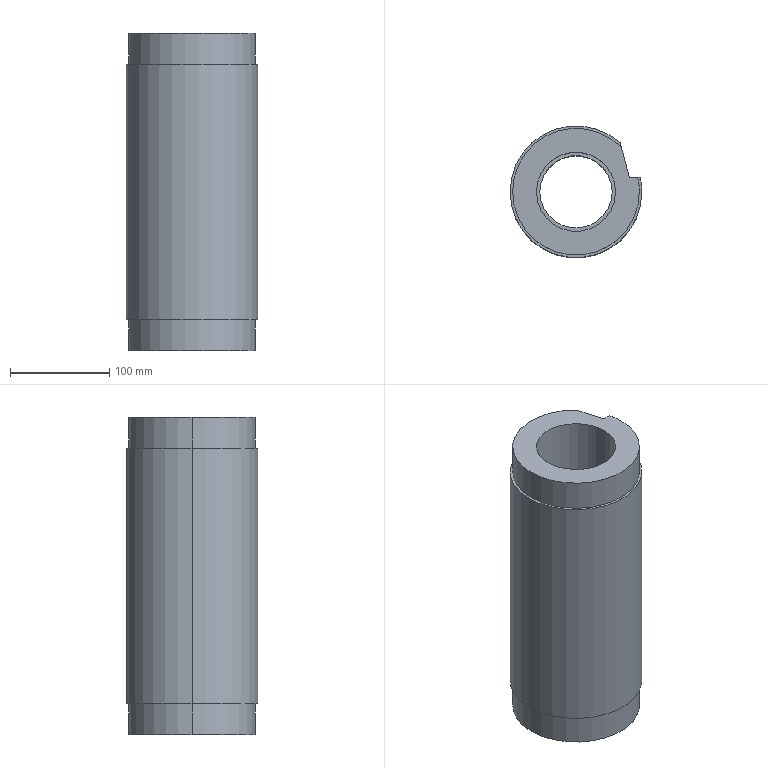Part | SolidWorks | features ICE 3, Extrusion 1, MirrorPattern 1 | 1 solid | 23 faces | box 133 x 133 x 320 mm | volume 2826163 mm3 | cylinder 15 | plane 8 | commonest cylinder face diameters 128 x6 80 x4 133 x3 73 x2
STEP:
#1=CARTESIAN_POINT('',(64.,0.,31.));
#2=VERTEX_POINT('',#1);
#3=CARTESIAN_POINT('',(62.336,14.5,31.));
#4=VERTEX_POINT('',#3);
#5=CARTESIAN_POINT('',(0.,0.,31.));
#6=DIRECTION('',(0.,0.,1.));
#7=DIRECTION('',(1.,0.,0.));
#8=AXIS2_PLACEMENT_3D('',#5,#6,#7);
#9=CIRCLE('',#8,64.);
#10=EDGE_CURVE('',#2,#4,#9,.T.);
#11=ORIENTED_EDGE('',*,*,#10,.F.);
#12=CARTESIAN_POINT('',(64.,0.,0.));
#13=VERTEX_POINT('',#12);
#14=CARTESIAN_POINT('',(64.,0.,31.));
#15=DIRECTION('',(0.,0.,-1.));
#16=VECTOR('',#15,1000.);
#17=LINE('',#14,#16);
#18=EDGE_CURVE('',#2,#13,#17,.T.);
#19=ORIENTED_EDGE('',*,*,#18,.T.);
#20=CARTESIAN_POINT('',(62.336,14.5,0.));
#21=VERTEX_POINT('',#20);
#22=CARTESIAN_POINT('',(0.,0.,0.));
#23=DIRECTION('',(0.,0.,1.));
#24=DIRECTION('',(1.,0.,0.));
#25=AXIS2_PLACEMENT_3D('',#22,#23,#24);
#26=CIRCLE('',#25,64.);
#27=EDGE_CURVE('',#13,#21,#26,.T.);
#28=ORIENTED_EDGE('',*,*,#27,.T.);
#29=CARTESIAN_POINT('',(62.336,14.5,31.));
#30=DIRECTION('',(0.,0.,1.));
#31=VECTOR('',#30,1000.);
#32=LINE('',#29,#31);
#33=EDGE_CURVE('',#21,#4,#32,.T.);
#34=ORIENTED_EDGE('',*,*,#33,.T.);
#35=EDGE_LOOP('',(#11,#19,#28,#34));
#36=FACE_OUTER_BOUND('',#35,.T.);
#37=CARTESIAN_POINT('',(0.,0.,31.));
#38=DIRECTION('',(0.,0.,-1.));
#39=DIRECTION('',(-1.,0.,0.));
#40=AXIS2_PLACEMENT_3D('',#37,#38,#39);
#41=CYLINDRICAL_SURFACE('',#40,64.);
#42=ADVANCED_FACE('',(#36),#41,.T.);
#43=ORIENTED_EDGE('',*,*,#18,.F.);
#44=CARTESIAN_POINT('',(-64.,0.,31.));
#45=VERTEX_POINT('',#44);
#46=CARTESIAN_POINT('',(0.,0.,31.));
#47=DIRECTION('',(0.,0.,1.));
#48=DIRECTION('',(1.,0.,0.));
#49=AXIS2_PLACEMENT_3D('',#46,#47,#48);
#50=CIRCLE('',#49,64.);
#51=EDGE_CURVE('',#45,#2,#50,.T.);
#52=ORIENTED_EDGE('',*,*,#51,.F.);
#53=CARTESIAN_POINT('',(-64.,0.,0.));
#54=VERTEX_POINT('',#53);
#55=CARTESIAN_POINT('',(-64.,0.,31.));
#56=DIRECTION('',(0.,0.,-1.));
#57=VECTOR('',#56,1000.);
#58=LINE('',#55,#57);
#59=EDGE_CURVE('',#45,#54,#58,.T.);
#60=ORIENTED_EDGE('',*,*,#59,.T.);
#61=CARTESIAN_POINT('',(0.,0.,0.));
#62=DIRECTION('',(0.,0.,1.));
#63=DIRECTION('',(1.,0.,0.));
#64=AXIS2_PLACEMENT_3D('',#61,#62,#63);
#65=CIRCLE('',#64,64.);
#66=EDGE_CURVE('',#54,#13,#65,.T.);
#67=ORIENTED_EDGE('',*,*,#66,.T.);
#68=EDGE_LOOP('',(#43,#52,#60,#67));
#69=FACE_OUTER_BOUND('',#68,.T.);
#70=CARTESIAN_POINT('',(0.,0.,31.));
#71=DIRECTION('',(0.,0.,-1.));
#72=DIRECTION('',(-1.,0.,0.));
#73=AXIS2_PLACEMENT_3D('',#70,#71,#72);
#74=CYLINDRICAL_SURFACE('',#73,64.);
#75=ADVANCED_FACE('',(#69),#74,.T.);
#76=CARTESIAN_POINT('',(-40.,0.,79.7));
#77=VERTEX_POINT('',#76);
#78=CARTESIAN_POINT('',(40.,0.,79.7));
#79=VERTEX_POINT('',#78);
#80=CARTESIAN_POINT('',(0.,0.,79.7));
#81=DIRECTION('',(0.,0.,1.));
#82=DIRECTION('',(1.,0.,0.));
#83=AXIS2_PLACEMENT_3D('',#80,#81,#82);
#84=CIRCLE('',#83,40.);
#85=EDGE_CURVE('',#77,#79,#84,.T.);
#86=ORIENTED_EDGE('',*,*,#85,.T.);
#87=CARTESIAN_POINT('',(40.,0.,0.));
#88=VERTEX_POINT('',#87);
#89=CARTESIAN_POINT('',(40.,0.,79.7));
#90=DIRECTION('',(0.,0.,-1.));
#91=VECTOR('',#90,1000.);
#92=LINE('',#89,#91);
#93=EDGE_CURVE('',#79,#88,#92,.T.);
#94=ORIENTED_EDGE('',*,*,#93,.T.);
#95=CARTESIAN_POINT('',(-40.,0.,0.));
#96=VERTEX_POINT('',#95);
#97=CARTESIAN_POINT('',(0.,0.,0.));
#98=DIRECTION('',(0.,0.,1.));
#99=DIRECTION('',(1.,0.,0.));
#100=AXIS2_PLACEMENT_3D('',#97,#98,#99);
#101=CIRCLE('',#100,40.);
#102=EDGE_CURVE('',#96,#88,#101,.T.);
#103=ORIENTED_EDGE('',*,*,#102,.F.);
#104=CARTESIAN_POINT('',(-40.,0.,79.7));
#105=DIRECTION('',(0.,0.,-1.));
#106=VECTOR('',#105,1000.);
#107=LINE('',#104,#106);
#108=EDGE_CURVE('',#77,#96,#107,.T.);
#109=ORIENTED_EDGE('',*,*,#108,.F.);
#110=EDGE_LOOP('',(#86,#94,#103,#109));
#111=FACE_OUTER_BOUND('',#110,.T.);
#112=CARTESIAN_POINT('',(0.,0.,79.7));
#113=DIRECTION('',(0.,0.,-1.));
#114=DIRECTION('',(-1.,0.,0.));
#115=AXIS2_PLACEMENT_3D('',#112,#113,#114);
#116=CYLINDRICAL_SURFACE('',#115,40.);
#117=ADVANCED_FACE('',(#111),#116,.F.);
#118=CARTESIAN_POINT('',(45.81,44.693,289.));
#119=VERTEX_POINT('',#118);
#120=CARTESIAN_POINT('',(-64.,0.,289.));
#121=VERTEX_POINT('',#120);
#122=CARTESIAN_POINT('',(0.,0.,289.));
#123=DIRECTION('',(0.,0.,1.));
#124=DIRECTION('',(1.,0.,0.));
#125=AXIS2_PLACEMENT_3D('',#122,#123,#124);
#126=CIRCLE('',#125,64.);
#127=EDGE_CURVE('',#119,#121,#126,.T.);
#128=ORIENTED_EDGE('',*,*,#127,.T.);
#129=CARTESIAN_POINT('',(-64.,0.,320.));
#130=VERTEX_POINT('',#129);
#131=CARTESIAN_POINT('',(-64.,0.,289.));
#132=DIRECTION('',(0.,0.,1.));
#133=VECTOR('',#132,1000.);
#134=LINE('',#131,#133);
#135=EDGE_CURVE('',#121,#130,#134,.T.);
#136=ORIENTED_EDGE('',*,*,#135,.T.);
#137=CARTESIAN_POINT('',(45.81,44.693,320.));
#138=VERTEX_POINT('',#137);
#139=CARTESIAN_POINT('',(0.,0.,320.));
#140=DIRECTION('',(0.,0.,1.));
#141=DIRECTION('',(1.,0.,0.));
#142=AXIS2_PLACEMENT_3D('',#139,#140,#141);
#143=CIRCLE('',#142,64.);
#144=EDGE_CURVE('',#138,#130,#143,.T.);
#145=ORIENTED_EDGE('',*,*,#144,.F.);
#146=CARTESIAN_POINT('',(45.81,44.693,289.));
#147=DIRECTION('',(0.,0.,1.));
#148=VECTOR('',#147,1000.);
#149=LINE('',#146,#148);
#150=EDGE_CURVE('',#119,#138,#149,.T.);
#151=ORIENTED_EDGE('',*,*,#150,.F.);
#152=EDGE_LOOP('',(#128,#136,#145,#151));
#153=FACE_OUTER_BOUND('',#152,.T.);
#154=CARTESIAN_POINT('',(0.,0.,289.));
#155=DIRECTION('',(0.,0.,1.));
#156=DIRECTION('',(1.,0.,0.));
#157=AXIS2_PLACEMENT_3D('',#154,#155,#156);
#158=CYLINDRICAL_SURFACE('',#157,64.);
#159=ADVANCED_FACE('',(#153),#158,.T.);
#160=ORIENTED_EDGE('',*,*,#135,.F.);
#161=CARTESIAN_POINT('',(64.,0.,289.));
#162=VERTEX_POINT('',#161);
#163=CARTESIAN_POINT('',(0.,0.,289.));
#164=DIRECTION('',(0.,0.,1.));
#165=DIRECTION('',(1.,0.,0.));
#166=AXIS2_PLACEMENT_3D('',#163,#164,#165);
#167=CIRCLE('',#166,64.);
#168=EDGE_CURVE('',#121,#162,#167,.T.);
#169=ORIENTED_EDGE('',*,*,#168,.T.);
#170=CARTESIAN_POINT('',(64.,0.,320.));
#171=VERTEX_POINT('',#170);
#172=CARTESIAN_POINT('',(64.,0.,289.));
#173=DIRECTION('',(0.,0.,1.));
#174=VECTOR('',#173,1000.);
#175=LINE('',#172,#174);
#176=EDGE_CURVE('',#162,#171,#175,.T.);
#177=ORIENTED_EDGE('',*,*,#176,.T.);
#178=CARTESIAN_POINT('',(0.,0.,320.));
#179=DIRECTION('',(0.,0.,1.));
#180=DIRECTION('',(1.,0.,0.));
#181=AXIS2_PLACEMENT_3D('',#178,#179,#180);
#182=CIRCLE('',#181,64.);
#183=EDGE_CURVE('',#130,#171,#182,.T.);
#184=ORIENTED_EDGE('',*,*,#183,.F.);
#185=EDGE_LOOP('',(#160,#169,#177,#184));
#186=FACE_OUTER_BOUND('',#185,.T.);
#187=CARTESIAN_POINT('',(0.,0.,289.));
#188=DIRECTION('',(0.,0.,1.));
#189=DIRECTION('',(1.,0.,0.));
#190=AXIS2_PLACEMENT_3D('',#187,#188,#189);
#191=CYLINDRICAL_SURFACE('',#190,64.);
#192=ADVANCED_FACE('',(#186),#191,.T.);
#193=CARTESIAN_POINT('',(-40.,0.,240.3));
#194=VERTEX_POINT('',#193);
#195=CARTESIAN_POINT('',(40.,0.,240.3));
#196=VERTEX_POINT('',#195);
#197=CARTESIAN_POINT('',(0.,0.,240.3));
#198=DIRECTION('',(0.,0.,1.));
#199=DIRECTION('',(1.,0.,0.));
#200=AXIS2_PLACEMENT_3D('',#197,#198,#199);
#201=CIRCLE('',#200,40.);
#202=EDGE_CURVE('',#194,#196,#201,.T.);
#203=ORIENTED_EDGE('',*,*,#202,.F.);
#204=CARTESIAN_POINT('',(-40.,0.,320.));
#205=VERTEX_POINT('',#204);
#206=CARTESIAN_POINT('',(-40.,0.,240.3));
#207=DIRECTION('',(0.,0.,1.));
#208=VECTOR('',#207,1000.);
#209=LINE('',#206,#208);
#210=EDGE_CURVE('',#194,#205,#209,.T.);
#211=ORIENTED_EDGE('',*,*,#210,.T.);
#212=CARTESIAN_POINT('',(40.,0.,320.));
#213=VERTEX_POINT('',#212);
#214=CARTESIAN_POINT('',(0.,0.,320.));
#215=DIRECTION('',(0.,0.,1.));
#216=DIRECTION('',(1.,0.,0.));
#217=AXIS2_PLACEMENT_3D('',#214,#215,#216);
#218=CIRCLE('',#217,40.);
#219=EDGE_CURVE('',#205,#213,#218,.T.);
#220=ORIENTED_EDGE('',*,*,#219,.T.);
#221=CARTESIAN_POINT('',(40.,0.,240.3));
#222=DIRECTION('',(0.,0.,1.));
#223=VECTOR('',#222,1000.);
#224=LINE('',#221,#223);
#225=EDGE_CURVE('',#196,#213,#224,.T.);
#226=ORIENTED_EDGE('',*,*,#225,.F.);
#227=EDGE_LOOP('',(#203,#211,#220,#226));
#228=FACE_OUTER_BOUND('',#227,.T.);
#229=CARTESIAN_POINT('',(0.,0.,240.3));
#230=DIRECTION('',(0.,0.,1.));
#231=DIRECTION('',(1.,0.,0.));
#232=AXIS2_PLACEMENT_3D('',#229,#230,#231);
#233=CYLINDRICAL_SURFACE('',#232,40.);
#234=ADVANCED_FACE('',(#228),#233,.F.);
#235=CARTESIAN_POINT('',(-36.5,0.,240.3));
#236=VERTEX_POINT('',#235);
#237=CARTESIAN_POINT('',(36.5,0.,240.3));
#238=VERTEX_POINT('',#237);
#239=CARTESIAN_POINT('',(0.,0.,240.3));
#240=DIRECTION('',(0.,0.,1.));
#241=DIRECTION('',(1.,0.,0.));
#242=AXIS2_PLACEMENT_3D('',#239,#240,#241);
#243=CIRCLE('',#242,36.5);
#244=EDGE_CURVE('',#236,#238,#243,.T.);
#245=ORIENTED_EDGE('',*,*,#244,.T.);
#246=CARTESIAN_POINT('',(36.5,0.,79.7));
#247=VERTEX_POINT('',#246);
#248=CARTESIAN_POINT('',(36.5,0.,320.));
#249=DIRECTION('',(0.,0.,-1.));
#250=VECTOR('',#249,1000.);
#251=LINE('',#248,#250);
#252=EDGE_CURVE('',#238,#247,#251,.T.);
#253=ORIENTED_EDGE('',*,*,#252,.T.);
#254=CARTESIAN_POINT('',(-36.5,0.,79.7));
#255=VERTEX_POINT('',#254);
#256=CARTESIAN_POINT('',(0.,0.,79.7));
#257=DIRECTION('',(0.,0.,-1.));
#258=DIRECTION('',(-1.,0.,0.));
#259=AXIS2_PLACEMENT_3D('',#256,#257,#258);
#260=CIRCLE('',#259,36.5);
#261=EDGE_CURVE('',#247,#255,#260,.T.);
#262=ORIENTED_EDGE('',*,*,#261,.T.);
#263=CARTESIAN_POINT('',(-36.5,0.,320.));
#264=DIRECTION('',(0.,0.,-1.));
#265=VECTOR('',#264,1000.);
#266=LINE('',#263,#265);
#267=EDGE_CURVE('',#236,#255,#266,.T.);
#268=ORIENTED_EDGE('',*,*,#267,.F.);
#269=EDGE_LOOP('',(#245,#253,#262,#268));
#270=FACE_OUTER_BOUND('',#269,.T.);
#271=CARTESIAN_POINT('',(0.,0.,320.));
#272=DIRECTION('',(0.,0.,-1.));
#273=DIRECTION('',(-1.,0.,0.));
#274=AXIS2_PLACEMENT_3D('',#271,#272,#273);
#275=CYLINDRICAL_SURFACE('',#274,36.5);
#276=ADVANCED_FACE('',(#270),#275,.F.);
#277=CARTESIAN_POINT('',(66.5,0.,289.));
#278=VERTEX_POINT('',#277);
#279=CARTESIAN_POINT('',(64.9,14.5,289.));
#280=VERTEX_POINT('',#279);
#281=CARTESIAN_POINT('',(0.,0.,289.));
#282=DIRECTION('',(0.,0.,1.));
#283=DIRECTION('',(1.,0.,0.));
#284=AXIS2_PLACEMENT_3D('',#281,#282,#283);
#285=CIRCLE('',#284,66.5);
#286=EDGE_CURVE('',#278,#280,#285,.T.);
#287=ORIENTED_EDGE('',*,*,#286,.F.);
#288=CARTESIAN_POINT('',(66.5,0.,31.));
#289=VERTEX_POINT('',#288);
#290=CARTESIAN_POINT('',(66.5,0.,320.));
#291=DIRECTION('',(0.,0.,-1.));
#292=VECTOR('',#291,1000.);
#293=LINE('',#290,#292);
#294=EDGE_CURVE('',#278,#289,#293,.T.);
#295=ORIENTED_EDGE('',*,*,#294,.T.);
#296=CARTESIAN_POINT('',(64.9,14.5,31.));
#297=VERTEX_POINT('',#296);
#298=CARTESIAN_POINT('',(0.,0.,31.));
#299=DIRECTION('',(0.,0.,1.));
#300=DIRECTION('',(1.,0.,0.));
#301=AXIS2_PLACEMENT_3D('',#298,#299,#300);
#302=CIRCLE('',#301,66.5);
#303=EDGE_CURVE('',#289,#297,#302,.T.);
#304=ORIENTED_EDGE('',*,*,#303,.T.);
#305=CARTESIAN_POINT('',(64.9,14.5,0.));
#306=DIRECTION('',(0.,0.,1.));
#307=VECTOR('',#306,1000.);
#308=LINE('',#305,#307);
#309=EDGE_CURVE('',#297,#280,#308,.T.);
#310=ORIENTED_EDGE('',*,*,#309,.T.);
#311=EDGE_LOOP('',(#287,#295,#304,#310));
#312=FACE_OUTER_BOUND('',#311,.T.);
#313=CARTESIAN_POINT('',(0.,0.,320.));
#314=DIRECTION('',(0.,0.,-1.));
#315=DIRECTION('',(-1.,0.,0.));
#316=AXIS2_PLACEMENT_3D('',#313,#314,#315);
#317=CYLINDRICAL_SURFACE('',#316,66.5);
#318=ADVANCED_FACE('',(#312),#317,.T.);
#319=ORIENTED_EDGE('',*,*,#294,.F.);
#320=CARTESIAN_POINT('',(-66.5,0.,289.));
#321=VERTEX_POINT('',#320);
#322=CARTESIAN_POINT('',(0.,0.,289.));
#323=DIRECTION('',(0.,0.,1.));
#324=DIRECTION('',(1.,0.,0.));
#325=AXIS2_PLACEMENT_3D('',#322,#323,#324);
#326=CIRCLE('',#325,66.5);
#327=EDGE_CURVE('',#321,#278,#326,.T.);
#328=ORIENTED_EDGE('',*,*,#327,.F.);
#329=CARTESIAN_POINT('',(-66.5,0.,31.));
#330=VERTEX_POINT('',#329);
#331=CARTESIAN_POINT('',(-66.5,0.,320.));
#332=DIRECTION('',(0.,0.,-1.));
#333=VECTOR('',#332,1000.);
#334=LINE('',#331,#333);
#335=EDGE_CURVE('',#321,#330,#334,.T.);
#336=ORIENTED_EDGE('',*,*,#335,.T.);
#337=CARTESIAN_POINT('',(0.,0.,31.));
#338=DIRECTION('',(0.,0.,1.));
#339=DIRECTION('',(1.,0.,0.));
#340=AXIS2_PLACEMENT_3D('',#337,#338,#339);
#341=CIRCLE('',#340,66.5);
#342=EDGE_CURVE('',#330,#289,#341,.T.);
#343=ORIENTED_EDGE('',*,*,#342,.T.);
#344=EDGE_LOOP('',(#319,#328,#336,#343));
#345=FACE_OUTER_BOUND('',#344,.T.);
#346=CARTESIAN_POINT('',(0.,0.,320.));
#347=DIRECTION('',(0.,0.,-1.));
#348=DIRECTION('',(-1.,0.,0.));
#349=AXIS2_PLACEMENT_3D('',#346,#347,#348);
#350=CYLINDRICAL_SURFACE('',#349,66.5);
#351=ADVANCED_FACE('',(#345),#350,.T.);
#352=ORIENTED_EDGE('',*,*,#335,.F.);
#353=CARTESIAN_POINT('',(44.558,49.364,289.));
#354=VERTEX_POINT('',#353);
#355=CARTESIAN_POINT('',(0.,0.,289.));
#356=DIRECTION('',(0.,0.,1.));
#357=DIRECTION('',(1.,0.,0.));
#358=AXIS2_PLACEMENT_3D('',#355,#356,#357);
#359=CIRCLE('',#358,66.5);
#360=EDGE_CURVE('',#354,#321,#359,.T.);
#361=ORIENTED_EDGE('',*,*,#360,.F.);
#362=CARTESIAN_POINT('',(44.558,49.364,31.));
#363=VERTEX_POINT('',#362);
#364=CARTESIAN_POINT('',(44.558,49.364,0.));
#365=DIRECTION('',(0.,0.,1.));
#366=VECTOR('',#365,1000.);
#367=LINE('',#364,#366);
#368=EDGE_CURVE('',#363,#354,#367,.T.);
#369=ORIENTED_EDGE('',*,*,#368,.F.);
#370=CARTESIAN_POINT('',(0.,0.,31.));
#371=DIRECTION('',(0.,0.,1.));
#372=DIRECTION('',(1.,0.,0.));
#373=AXIS2_PLACEMENT_3D('',#370,#371,#372);
#374=CIRCLE('',#373,66.5);
#375=EDGE_CURVE('',#363,#330,#374,.T.);
#376=ORIENTED_EDGE('',*,*,#375,.T.);
#377=EDGE_LOOP('',(#352,#361,#369,#376));
#378=FACE_OUTER_BOUND('',#377,.T.);
#379=CARTESIAN_POINT('',(0.,0.,320.));
#380=DIRECTION('',(0.,0.,-1.));
#381=DIRECTION('',(-1.,0.,0.));
#382=AXIS2_PLACEMENT_3D('',#379,#380,#381);
#383=CYLINDRICAL_SURFACE('',#382,66.5);
#384=ADVANCED_FACE('',(#378),#383,.T.);
#385=ORIENTED_EDGE('',*,*,#252,.F.);
#386=CARTESIAN_POINT('',(0.,0.,240.3));
#387=DIRECTION('',(0.,0.,1.));
#388=DIRECTION('',(1.,0.,0.));
#389=AXIS2_PLACEMENT_3D('',#386,#387,#388);
#390=CIRCLE('',#389,36.5);
#391=EDGE_CURVE('',#238,#236,#390,.T.);
#392=ORIENTED_EDGE('',*,*,#391,.T.);
#393=ORIENTED_EDGE('',*,*,#267,.T.);
#394=CARTESIAN_POINT('',(0.,0.,79.7));
#395=DIRECTION('',(0.,0.,-1.));
#396=DIRECTION('',(-1.,0.,0.));
#397=AXIS2_PLACEMENT_3D('',#394,#395,#396);
#398=CIRCLE('',#397,36.5);
#399=EDGE_CURVE('',#255,#247,#398,.T.);
#400=ORIENTED_EDGE('',*,*,#399,.T.);
#401=EDGE_LOOP('',(#385,#392,#393,#400));
#402=FACE_OUTER_BOUND('',#401,.T.);
#403=CARTESIAN_POINT('',(0.,0.,320.));
#404=DIRECTION('',(0.,0.,-1.));
#405=DIRECTION('',(-1.,0.,0.));
#406=AXIS2_PLACEMENT_3D('',#403,#404,#405);
#407=CYLINDRICAL_SURFACE('',#406,36.5);
#408=ADVANCED_FACE('',(#402),#407,.F.);
#409=CARTESIAN_POINT('',(45.81,44.693,0.));
#410=VERTEX_POINT('',#409);
#411=CARTESIAN_POINT('',(53.9,14.5,0.));
#412=VERTEX_POINT('',#411);
#413=CARTESIAN_POINT('',(53.9,14.5,0.));
#414=DIRECTION('',(0.2588,-0.9659,0.));
#415=VECTOR('',#414,1000.);
#416=LINE('',#413,#415);
#417=EDGE_CURVE('',#410,#412,#416,.T.);
#418=ORIENTED_EDGE('',*,*,#417,.T.);
#419=CARTESIAN_POINT('',(64.9,14.5,0.));
#420=DIRECTION('',(1.,0.,0.));
#421=VECTOR('',#420,1000.);
#422=LINE('',#419,#421);
#423=EDGE_CURVE('',#412,#21,#422,.T.);
#424=ORIENTED_EDGE('',*,*,#423,.T.);
#425=ORIENTED_EDGE('',*,*,#27,.F.);
#426=ORIENTED_EDGE('',*,*,#66,.F.);
#427=CARTESIAN_POINT('',(0.,0.,0.));
#428=DIRECTION('',(0.,0.,1.));
#429=DIRECTION('',(1.,0.,0.));
#430=AXIS2_PLACEMENT_3D('',#427,#428,#429);
#431=CIRCLE('',#430,64.);
#432=EDGE_CURVE('',#410,#54,#431,.T.);
#433=ORIENTED_EDGE('',*,*,#432,.F.);
#434=EDGE_LOOP('',(#418,#424,#425,#426,#433));
#435=FACE_OUTER_BOUND('',#434,.T.);
#436=ORIENTED_EDGE('',*,*,#102,.T.);
#437=CARTESIAN_POINT('',(0.,0.,0.));
#438=DIRECTION('',(0.,0.,1.));
#439=DIRECTION('',(1.,0.,0.));
#440=AXIS2_PLACEMENT_3D('',#437,#438,#439);
#441=CIRCLE('',#440,40.);
#442=EDGE_CURVE('',#88,#96,#441,.T.);
#443=ORIENTED_EDGE('',*,*,#442,.T.);
#444=EDGE_LOOP('',(#436,#443));
#445=FACE_BOUND('',#444,.T.);
#446=CARTESIAN_POINT('',(0.,0.,0.));
#447=DIRECTION('',(0.,0.,1.));
#448=DIRECTION('',(1.,0.,0.));
#449=AXIS2_PLACEMENT_3D('',#446,#447,#448);
#450=PLANE('',#449);
#451=ADVANCED_FACE('',(#435,#445),#450,.F.);
#452=CARTESIAN_POINT('',(53.9,14.5,320.));
#453=VERTEX_POINT('',#452);
#454=CARTESIAN_POINT('',(62.336,14.5,320.));
#455=VERTEX_POINT('',#454);
#456=CARTESIAN_POINT('',(64.9,14.5,320.));
#457=DIRECTION('',(1.,0.,0.));
#458=VECTOR('',#457,1000.);
#459=LINE('',#456,#458);
#460=EDGE_CURVE('',#453,#455,#459,.T.);
#461=ORIENTED_EDGE('',*,*,#460,.F.);
#462=CARTESIAN_POINT('',(53.9,14.5,320.));
#463=DIRECTION('',(0.2588,-0.9659,0.));
#464=VECTOR('',#463,1000.);
#465=LINE('',#462,#464);
#466=EDGE_CURVE('',#138,#453,#465,.T.);
#467=ORIENTED_EDGE('',*,*,#466,.F.);
#468=ORIENTED_EDGE('',*,*,#144,.T.);
#469=ORIENTED_EDGE('',*,*,#183,.T.);
#470=CARTESIAN_POINT('',(0.,0.,320.));
#471=DIRECTION('',(0.,0.,1.));
#472=DIRECTION('',(1.,0.,0.));
#473=AXIS2_PLACEMENT_3D('',#470,#471,#472);
#474=CIRCLE('',#473,64.);
#475=EDGE_CURVE('',#171,#455,#474,.T.);
#476=ORIENTED_EDGE('',*,*,#475,.T.);
#477=EDGE_LOOP('',(#461,#467,#468,#469,#476));
#478=FACE_OUTER_BOUND('',#477,.T.);
#479=CARTESIAN_POINT('',(0.,0.,320.));
#480=DIRECTION('',(0.,0.,1.));
#481=DIRECTION('',(1.,0.,0.));
#482=AXIS2_PLACEMENT_3D('',#479,#480,#481);
#483=CIRCLE('',#482,40.);
#484=EDGE_CURVE('',#213,#205,#483,.T.);
#485=ORIENTED_EDGE('',*,*,#484,.F.);
#486=ORIENTED_EDGE('',*,*,#219,.F.);
#487=EDGE_LOOP('',(#485,#486));
#488=FACE_BOUND('',#487,.T.);
#489=CARTESIAN_POINT('',(0.,0.,320.));
#490=DIRECTION('',(0.,0.,1.));
#491=DIRECTION('',(1.,0.,0.));
#492=AXIS2_PLACEMENT_3D('',#489,#490,#491);
#493=PLANE('',#492);
#494=ADVANCED_FACE('',(#478,#488),#493,.T.);
#495=ORIENTED_EDGE('',*,*,#210,.F.);
#496=CARTESIAN_POINT('',(0.,0.,240.3));
#497=DIRECTION('',(0.,0.,1.));
#498=DIRECTION('',(1.,0.,0.));
#499=AXIS2_PLACEMENT_3D('',#496,#497,#498);
#500=CIRCLE('',#499,40.);
#501=EDGE_CURVE('',#196,#194,#500,.T.);
#502=ORIENTED_EDGE('',*,*,#501,.F.);
#503=ORIENTED_EDGE('',*,*,#225,.T.);
#504=ORIENTED_EDGE('',*,*,#484,.T.);
#505=EDGE_LOOP('',(#495,#502,#503,#504));
#506=FACE_OUTER_BOUND('',#505,.T.);
#507=CARTESIAN_POINT('',(0.,0.,240.3));
#508=DIRECTION('',(0.,0.,1.));
#509=DIRECTION('',(1.,0.,0.));
#510=AXIS2_PLACEMENT_3D('',#507,#508,#509);
#511=CYLINDRICAL_SURFACE('',#510,40.);
#512=ADVANCED_FACE('',(#506),#511,.F.);
#513=ORIENTED_EDGE('',*,*,#244,.F.);
#514=ORIENTED_EDGE('',*,*,#391,.F.);
#515=EDGE_LOOP('',(#513,#514));
#516=FACE_BOUND('',#515,.T.);
#517=ORIENTED_EDGE('',*,*,#501,.T.);
#518=ORIENTED_EDGE('',*,*,#202,.T.);
#519=EDGE_LOOP('',(#517,#518));
#520=FACE_OUTER_BOUND('',#519,.T.);
#521=CARTESIAN_POINT('',(0.,0.,240.3));
#522=DIRECTION('',(0.,0.,1.));
#523=DIRECTION('',(1.,0.,0.));
#524=AXIS2_PLACEMENT_3D('',#521,#522,#523);
#525=PLANE('',#524);
#526=ADVANCED_FACE('',(#516,#520),#525,.T.);
#527=CARTESIAN_POINT('',(62.336,14.5,289.));
#528=VERTEX_POINT('',#527);
#529=CARTESIAN_POINT('',(0.,14.5,289.));
#530=DIRECTION('',(1.,0.,0.));
#531=VECTOR('',#530,1000.);
#532=LINE('',#529,#531);
#533=EDGE_CURVE('',#528,#280,#532,.T.);
#534=ORIENTED_EDGE('',*,*,#533,.F.);
#535=CARTESIAN_POINT('',(0.,0.,289.));
#536=DIRECTION('',(0.,0.,1.));
#537=DIRECTION('',(1.,0.,0.));
#538=AXIS2_PLACEMENT_3D('',#535,#536,#537);
#539=CIRCLE('',#538,64.);
#540=EDGE_CURVE('',#162,#528,#539,.T.);
#541=ORIENTED_EDGE('',*,*,#540,.F.);
#542=ORIENTED_EDGE('',*,*,#168,.F.);
#543=ORIENTED_EDGE('',*,*,#127,.F.);
#544=CARTESIAN_POINT('',(53.914,14.446,289.));
#545=DIRECTION('',(0.2588,-0.9659,0.));
#546=VECTOR('',#545,1000.);
#547=LINE('',#544,#546);
#548=EDGE_CURVE('',#354,#119,#547,.T.);
#549=ORIENTED_EDGE('',*,*,#548,.F.);
#550=ORIENTED_EDGE('',*,*,#360,.T.);
#551=ORIENTED_EDGE('',*,*,#327,.T.);
#552=ORIENTED_EDGE('',*,*,#286,.T.);
#553=EDGE_LOOP('',(#534,#541,#542,#543,#549,#550,#551,#552));
#554=FACE_OUTER_BOUND('',#553,.T.);
#555=CARTESIAN_POINT('',(0.,0.,289.));
#556=DIRECTION('',(0.,0.,1.));
#557=DIRECTION('',(1.,0.,0.));
#558=AXIS2_PLACEMENT_3D('',#555,#556,#557);
#559=PLANE('',#558);
#560=ADVANCED_FACE('',(#554),#559,.T.);
#561=ORIENTED_EDGE('',*,*,#176,.F.);
#562=ORIENTED_EDGE('',*,*,#540,.T.);
#563=CARTESIAN_POINT('',(62.336,14.5,289.));
#564=DIRECTION('',(0.,0.,-1.));
#565=VECTOR('',#564,1000.);
#566=LINE('',#563,#565);
#567=EDGE_CURVE('',#455,#528,#566,.T.);
#568=ORIENTED_EDGE('',*,*,#567,.F.);
#569=ORIENTED_EDGE('',*,*,#475,.F.);
#570=EDGE_LOOP('',(#561,#562,#568,#569));
#571=FACE_OUTER_BOUND('',#570,.T.);
#572=CARTESIAN_POINT('',(0.,0.,289.));
#573=DIRECTION('',(0.,0.,1.));
#574=DIRECTION('',(1.,0.,0.));
#575=AXIS2_PLACEMENT_3D('',#572,#573,#574);
#576=CYLINDRICAL_SURFACE('',#575,64.);
#577=ADVANCED_FACE('',(#571),#576,.T.);
#578=ORIENTED_EDGE('',*,*,#93,.F.);
#579=CARTESIAN_POINT('',(0.,0.,79.7));
#580=DIRECTION('',(0.,0.,1.));
#581=DIRECTION('',(1.,0.,0.));
#582=AXIS2_PLACEMENT_3D('',#579,#580,#581);
#583=CIRCLE('',#582,40.);
#584=EDGE_CURVE('',#79,#77,#583,.T.);
#585=ORIENTED_EDGE('',*,*,#584,.T.);
#586=ORIENTED_EDGE('',*,*,#108,.T.);
#587=ORIENTED_EDGE('',*,*,#442,.F.);
#588=EDGE_LOOP('',(#578,#585,#586,#587));
#589=FACE_OUTER_BOUND('',#588,.T.);
#590=CARTESIAN_POINT('',(0.,0.,79.7));
#591=DIRECTION('',(0.,0.,-1.));
#592=DIRECTION('',(-1.,0.,0.));
#593=AXIS2_PLACEMENT_3D('',#590,#591,#592);
#594=CYLINDRICAL_SURFACE('',#593,40.);
#595=ADVANCED_FACE('',(#589),#594,.F.);
#596=ORIENTED_EDGE('',*,*,#399,.F.);
#597=ORIENTED_EDGE('',*,*,#261,.F.);
#598=EDGE_LOOP('',(#596,#597));
#599=FACE_BOUND('',#598,.T.);
#600=ORIENTED_EDGE('',*,*,#85,.F.);
#601=ORIENTED_EDGE('',*,*,#584,.F.);
#602=EDGE_LOOP('',(#600,#601));
#603=FACE_OUTER_BOUND('',#602,.T.);
#604=CARTESIAN_POINT('',(0.,0.,79.7));
#605=DIRECTION('',(0.,0.,-1.));
#606=DIRECTION('',(1.,0.,0.));
#607=AXIS2_PLACEMENT_3D('',#604,#605,#606);
#608=PLANE('',#607);
#609=ADVANCED_FACE('',(#599,#603),#608,.T.);
#610=CARTESIAN_POINT('',(0.,14.5,31.));
#611=DIRECTION('',(-1.,0.,0.));
#612=VECTOR('',#611,1000.);
#613=LINE('',#610,#612);
#614=EDGE_CURVE('',#297,#4,#613,.T.);
#615=ORIENTED_EDGE('',*,*,#614,.F.);
#616=ORIENTED_EDGE('',*,*,#303,.F.);
#617=ORIENTED_EDGE('',*,*,#342,.F.);
#618=ORIENTED_EDGE('',*,*,#375,.F.);
#619=CARTESIAN_POINT('',(45.81,44.693,31.));
#620=VERTEX_POINT('',#619);
#621=CARTESIAN_POINT('',(53.914,14.446,31.));
#622=DIRECTION('',(-0.2588,0.9659,0.));
#623=VECTOR('',#622,1000.);
#624=LINE('',#621,#623);
#625=EDGE_CURVE('',#620,#363,#624,.T.);
#626=ORIENTED_EDGE('',*,*,#625,.F.);
#627=CARTESIAN_POINT('',(0.,0.,31.));
#628=DIRECTION('',(0.,0.,1.));
#629=DIRECTION('',(1.,0.,0.));
#630=AXIS2_PLACEMENT_3D('',#627,#628,#629);
#631=CIRCLE('',#630,64.);
#632=EDGE_CURVE('',#620,#45,#631,.T.);
#633=ORIENTED_EDGE('',*,*,#632,.T.);
#634=ORIENTED_EDGE('',*,*,#51,.T.);
#635=ORIENTED_EDGE('',*,*,#10,.T.);
#636=EDGE_LOOP('',(#615,#616,#617,#618,#626,#633,#634,#635));
#637=FACE_OUTER_BOUND('',#636,.T.);
#638=CARTESIAN_POINT('',(0.,0.,31.));
#639=DIRECTION('',(0.,0.,-1.));
#640=DIRECTION('',(1.,0.,0.));
#641=AXIS2_PLACEMENT_3D('',#638,#639,#640);
#642=PLANE('',#641);
#643=ADVANCED_FACE('',(#637),#642,.T.);
#644=ORIENTED_EDGE('',*,*,#59,.F.);
#645=ORIENTED_EDGE('',*,*,#632,.F.);
#646=CARTESIAN_POINT('',(45.81,44.693,31.));
#647=DIRECTION('',(0.,0.,-1.));
#648=VECTOR('',#647,1000.);
#649=LINE('',#646,#648);
#650=EDGE_CURVE('',#620,#410,#649,.T.);
#651=ORIENTED_EDGE('',*,*,#650,.T.);
#652=ORIENTED_EDGE('',*,*,#432,.T.);
#653=EDGE_LOOP('',(#644,#645,#651,#652));
#654=FACE_OUTER_BOUND('',#653,.T.);
#655=CARTESIAN_POINT('',(0.,0.,31.));
#656=DIRECTION('',(0.,0.,-1.));
#657=DIRECTION('',(-1.,0.,0.));
#658=AXIS2_PLACEMENT_3D('',#655,#656,#657);
#659=CYLINDRICAL_SURFACE('',#658,64.);
#660=ADVANCED_FACE('',(#654),#659,.T.);
#661=ORIENTED_EDGE('',*,*,#533,.T.);
#662=ORIENTED_EDGE('',*,*,#309,.F.);
#663=ORIENTED_EDGE('',*,*,#614,.T.);
#664=ORIENTED_EDGE('',*,*,#33,.F.);
#665=ORIENTED_EDGE('',*,*,#423,.F.);
#666=CARTESIAN_POINT('',(53.9,14.5,0.));
#667=DIRECTION('',(0.,0.,1.));
#668=VECTOR('',#667,1000.);
#669=LINE('',#666,#668);
#670=EDGE_CURVE('',#412,#453,#669,.T.);
#671=ORIENTED_EDGE('',*,*,#670,.T.);
#672=ORIENTED_EDGE('',*,*,#460,.T.);
#673=ORIENTED_EDGE('',*,*,#567,.T.);
#674=EDGE_LOOP('',(#661,#662,#663,#664,#665,#671,#672,#673));
#675=FACE_OUTER_BOUND('',#674,.T.);
#676=CARTESIAN_POINT('',(64.9,14.5,0.));
#677=DIRECTION('',(0.,-1.,0.));
#678=DIRECTION('',(0.,0.,-1.));
#679=AXIS2_PLACEMENT_3D('',#676,#677,#678);
#680=PLANE('',#679);
#681=ADVANCED_FACE('',(#675),#680,.F.);
#682=ORIENTED_EDGE('',*,*,#548,.T.);
#683=ORIENTED_EDGE('',*,*,#150,.T.);
#684=ORIENTED_EDGE('',*,*,#466,.T.);
#685=ORIENTED_EDGE('',*,*,#670,.F.);
#686=ORIENTED_EDGE('',*,*,#417,.F.);
#687=ORIENTED_EDGE('',*,*,#650,.F.);
#688=ORIENTED_EDGE('',*,*,#625,.T.);
#689=ORIENTED_EDGE('',*,*,#368,.T.);
#690=EDGE_LOOP('',(#682,#683,#684,#685,#686,#687,#688,#689));
#691=FACE_OUTER_BOUND('',#690,.T.);
#692=CARTESIAN_POINT('',(53.9,14.5,0.));
#693=DIRECTION('',(-0.9659,-0.2588,0.));
#694=DIRECTION('',(0.2588,-0.9659,0.));
#695=AXIS2_PLACEMENT_3D('',#692,#693,#694);
#696=PLANE('',#695);
#697=ADVANCED_FACE('',(#691),#696,.F.);
#698=CLOSED_SHELL('',(#42,#75,#117,#159,#192,#234,#276,#318,#351,#384,#408,#451,#494,#512,#526,#560,#577,#595,#609,#643,#660,#681,#697));
#699=MANIFOLD_SOLID_BREP('',#698);
#700=CARTESIAN_POINT('',(0.,0.,0.));
#701=DIRECTION('',(0.,0.,1.));
#702=DIRECTION('',(1.,0.,0.));
#703=AXIS2_PLACEMENT_3D('',#700,#701,#702);
#704=(LENGTH_UNIT()NAMED_UNIT(*)SI_UNIT(.MILLI.,.METRE.));
#705=UNCERTAINTY_MEASURE_WITH_UNIT(LENGTH_MEASURE(0.00001),#704,'','');
#706=(NAMED_UNIT(*)PLANE_ANGLE_UNIT()SI_UNIT($,.RADIAN.));
#707=(NAMED_UNIT(*)SI_UNIT($,.STERADIAN.)SOLID_ANGLE_UNIT());
#708=(GEOMETRIC_REPRESENTATION_CONTEXT(3)GLOBAL_UNCERTAINTY_ASSIGNED_CONTEXT((#705))GLOBAL_UNIT_ASSIGNED_CONTEXT((#704,#706,#707))REPRESENTATION_CONTEXT('',''));
#709=ADVANCED_BREP_SHAPE_REPRESENTATION('',(#699,#703),#708);